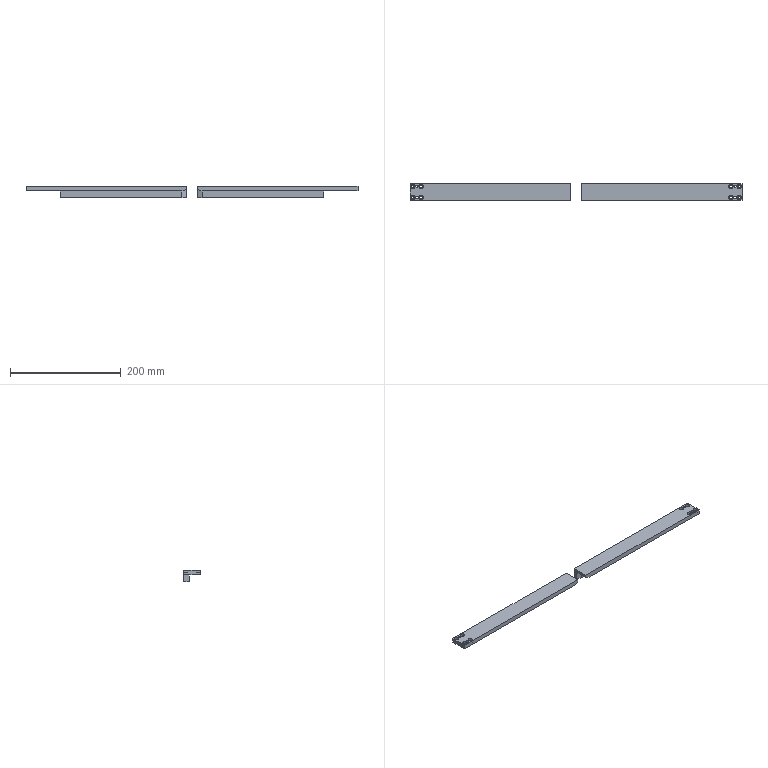NC program | NX | posted with a generic post | part box 600 x 30 x 20 mm
Lines 377 to 1170 of 2978:
(ZLEVEL_PROFILE_COPY_1_COPY , TOOL : D3)
N716 T20 M6
N718 G54
N720 G17 G0 G90 X-132.849 Y9.713 S7000 M3
N722 G43 Z30. H20
N724 Z1.
N726 G94 G1 X-132.821 Y9.67 Z0.997 F1000.
N728 X-132.617 Y9.555 Z0.985
N730 X-132.383 Z0.973
N732 X-132.179 Y9.67 Z0.961
N734 X-132.073 Y9.829 Z0.951
N736 X-132.04 Y10. Z0.941
N738 X-132.073 Y10.171 Z0.932
N740 X-132.179 Y10.33 Z0.922
N742 X-132.405 Y10.45 Z0.909
N744 X-132.595 Z0.899
N746 X-132.671 Y10.427 Z0.895
N748 X-132.83 Y10.321 Z0.885
N750 X-132.951 Y10.089 Z0.871
N752 X-132.927 Y9.829 Z0.857
N754 X-132.821 Y9.67 Z0.847
N756 X-132.617 Y9.555 Z0.835
N758 X-132.383 Z0.823
N760 X-132.179 Y9.67 Z0.811
N762 X-132.073 Y9.829 Z0.801
N764 X-132.04 Y10. Z0.791
N766 X-132.073 Y10.171 Z0.782
N768 X-132.179 Y10.33 Z0.772
N770 X-132.405 Y10.45 Z0.759
N772 X-132.595 Z0.749
N774 X-132.671 Y10.427 Z0.745
N776 X-132.83 Y10.321 Z0.735
N778 X-132.951 Y10.089 Z0.721
N780 X-132.927 Y9.829 Z0.707
N782 X-132.821 Y9.67 Z0.697
N784 X-132.617 Y9.555 Z0.685
N786 X-132.383 Z0.673
N788 X-132.179 Y9.67 Z0.66
N790 X-132.073 Y9.829 Z0.65
N792 X-132.04 Y10. Z0.641
N794 X-132.073 Y10.171 Z0.632
N796 X-132.179 Y10.33 Z0.622
N798 X-132.405 Y10.45 Z0.609
N800 X-132.595 Z0.599
N802 X-132.671 Y10.427 Z0.595
N804 X-132.83 Y10.321 Z0.585
N806 X-132.951 Y10.089 Z0.571
N808 X-132.927 Y9.829 Z0.557
N810 X-132.821 Y9.67 Z0.547
N812 X-132.617 Y9.555 Z0.535
N814 X-132.383 Z0.523
N816 X-132.179 Y9.67 Z0.51
N818 X-132.073 Y9.829 Z0.5
N820 X-132.04 Y10. Z0.491
N822 X-132.073 Y10.171 Z0.482
N824 X-132.179 Y10.33 Z0.472
N826 X-132.405 Y10.45 Z0.459
N828 X-132.595 Z0.449
N830 X-132.671 Y10.427 Z0.445
N832 X-132.83 Y10.321 Z0.435
N834 X-132.951 Y10.089 Z0.421
N836 X-132.927 Y9.829 Z0.407
N838 X-132.821 Y9.67 Z0.397
N840 X-132.617 Y9.555 Z0.385
N842 X-132.383 Z0.373
N844 X-132.179 Y9.67 Z0.36
N846 X-132.073 Y9.829 Z0.35
N848 X-132.04 Y10. Z0.341
N850 X-132.073 Y10.171 Z0.332
N852 X-132.179 Y10.33 Z0.322
N854 X-132.405 Y10.45 Z0.309
N856 X-132.595 Z0.299
N858 X-132.671 Y10.427 Z0.295
N860 X-132.83 Y10.321 Z0.285
N862 X-132.951 Y10.089 Z0.271
N864 X-132.927 Y9.829 Z0.257
N866 X-132.821 Y9.67 Z0.247
N868 X-132.617 Y9.555 Z0.235
N870 X-132.383 Z0.223
N872 X-132.179 Y9.67 Z0.21
N874 X-132.073 Y9.829 Z0.2
N876 X-132.04 Y10. Z0.191
N878 X-132.073 Y10.171 Z0.182
N880 X-132.179 Y10.33 Z0.172
N882 X-132.405 Y10.45 Z0.159
N884 X-132.595 Z0.149
N886 X-132.671 Y10.427 Z0.145
N888 X-132.83 Y10.321 Z0.135
N890 X-132.951 Y10.089 Z0.121
N892 X-132.927 Y9.829 Z0.107
N894 X-132.821 Y9.67 Z0.097
N896 X-132.617 Y9.555 Z0.085
N898 X-132.383 Z0.073
N900 X-132.179 Y9.67 Z0.06
N902 X-132.073 Y9.829 Z0.05
N904 X-132.04 Y10. Z0.041
N906 X-132.073 Y10.171 Z0.032
N908 X-132.179 Y10.33 Z0.022
N910 X-132.405 Y10.45 Z0.009
N912 X-132.595 Z-0.001
N914 X-132.671 Y10.427 Z-0.005
N916 X-132.83 Y10.321 Z-0.015
N918 X-132.951 Y10.089 Z-0.029
N920 X-132.927 Y9.829 Z-0.043
N922 X-132.821 Y9.67 Z-0.053
N924 X-132.617 Y9.555 Z-0.065
N926 X-132.383 Z-0.077
N928 X-132.179 Y9.67 Z-0.09
N930 X-132.073 Y9.829 Z-0.1
N932 X-132.04 Y10. Z-0.109
N934 X-132.073 Y10.171 Z-0.118
N936 X-132.179 Y10.33 Z-0.128
N938 X-132.405 Y10.45 Z-0.141
N940 X-132.595 Z-0.151
N942 X-132.671 Y10.427 Z-0.155
N944 X-132.83 Y10.321 Z-0.165
N946 X-132.951 Y10.089 Z-0.179
N948 X-132.927 Y9.829 Z-0.193
N950 X-132.821 Y9.67 Z-0.203
N952 X-132.617 Y9.555 Z-0.215
N954 X-132.383 Z-0.227
N956 X-132.179 Y9.67 Z-0.24
N958 X-132.073 Y9.829 Z-0.25
N960 X-132.04 Y10. Z-0.259
N962 X-132.073 Y10.171 Z-0.268
N964 X-132.179 Y10.33 Z-0.278
N966 X-132.405 Y10.45 Z-0.291
N968 X-132.5 Z-0.296
N970 G3 X-132.95 Y10. R0.45 F1300.
N972 X-132.5 Y10.45 R-0.45
N974 G1 X-132.596 Y10.433 Z-0.31
N976 X-132.669 Y10.41 Z-0.321
N978 X-132.721 Y10.383 Z-0.329
N980 X-132.8 Y10.325 Z-0.343
N982 X-132.851 Y10.269 Z-0.354
N984 X-132.883 Y10.221 Z-0.362
N986 X-132.921 Y10.132 Z-0.376
N988 X-132.936 Y10.086 Z-0.383
N990 X-132.944 Y10. Z-0.395
N992 X-132.933 Y9.91 Z-0.408
N994 X-132.911 Y9.837 Z-0.419
N996 X-132.883 Y9.779 Z-0.428
N998 X-132.828 Y9.702 Z-0.441
N1000 X-132.795 Y9.67 Z-0.448
N1002 X-132.771 Y9.651 Z-0.452
N1004 X-132.721 Y9.617 Z-0.461
N1006 X-132.632 Y9.579 Z-0.474
N1008 X-132.587 Y9.564 Z-0.481
N1010 X-132.5 Y9.556 Z-0.494
N1012 X-132.412 Y9.565 Z-0.506
N1014 X-132.339 Y9.587 Z-0.517
N1016 X-132.279 Y9.617 Z-0.527
N1018 X-132.197 Y9.678 Z-0.541
N1020 X-132.163 Y9.715 Z-0.548
N1022 X-132.11 Y9.775 Z-0.56
N1024 X-132.084 Y9.828 Z-0.568
N1026 X-132.065 Y9.884 Z-0.576
N1028 X-132.054 Y9.941 Z-0.584
N1030 X-132.05 Y10. Z-0.593
N1032 G3 X-132.5 Y10.45 R0.45
N1034 G1 X-132.596 Y10.433 Z-0.606
N1036 X-132.669 Y10.41 Z-0.617
N1038 X-132.721 Y10.383 Z-0.626
N1040 X-132.8 Y10.325 Z-0.639
N1042 X-132.851 Y10.269 Z-0.65
N1044 X-132.883 Y10.221 Z-0.658
N1046 X-132.921 Y10.132 Z-0.672
N1048 X-132.936 Y10.086 Z-0.679
N1050 X-132.944 Y10. Z-0.691
N1052 X-132.933 Y9.91 Z-0.704
N1054 X-132.911 Y9.837 Z-0.715
N1056 X-132.883 Y9.779 Z-0.724
N1058 X-132.827 Y9.702 Z-0.738
N1060 X-132.795 Y9.67 Z-0.744
N1062 X-132.771 Y9.651 Z-0.748
N1064 X-132.721 Y9.617 Z-0.757
N1066 X-132.632 Y9.579 Z-0.771
N1068 X-132.587 Y9.564 Z-0.778
N1070 X-132.5 Y9.556 Z-0.79
N1072 X-132.412 Y9.565 Z-0.803
N1074 X-132.339 Y9.587 Z-0.814
N1076 X-132.279 Y9.617 Z-0.823
N1078 X-132.197 Y9.678 Z-0.837
N1080 X-132.163 Y9.715 Z-0.845
N1082 X-132.11 Y9.775 Z-0.856
N1084 X-132.084 Y9.828 Z-0.864
N1086 X-132.065 Y9.884 Z-0.872
N1088 X-132.054 Y9.941 Z-0.881
N1090 X-132.05 Y10. Z-0.889
N1092 G3 X-132.5 Y10.45 R0.45
N1094 G1 X-132.596 Y10.433 Z-0.902
N1096 X-132.669 Y10.41 Z-0.913
N1098 X-132.721 Y10.383 Z-0.922
N1100 X-132.8 Y10.325 Z-0.936
N1102 X-132.851 Y10.269 Z-0.946
N1104 X-132.883 Y10.221 Z-0.955
N1106 X-132.921 Y10.132 Z-0.968
N1108 X-132.936 Y10.086 Z-0.975
N1110 X-132.944 Y10. Z-0.988
N1112 X-132.933 Y9.91 Z-1.
N1114 X-132.911 Y9.837 Z-1.011
N1116 X-132.883 Y9.779 Z-1.021
N1118 X-132.827 Y9.702 Z-1.034
N1120 X-132.795 Y9.67 Z-1.04
N1122 X-132.771 Y9.651 Z-1.045
N1124 X-132.721 Y9.617 Z-1.053
N1126 X-132.632 Y9.579 Z-1.067
N1128 X-132.587 Y9.564 Z-1.074
N1130 X-132.5 Y9.556 Z-1.086
N1132 X-132.412 Y9.565 Z-1.099
N1134 X-132.339 Y9.587 Z-1.11
N1136 X-132.279 Y9.617 Z-1.119
N1138 X-132.197 Y9.678 Z-1.134
N1140 X-132.163 Y9.715 Z-1.141
N1142 X-132.11 Y9.775 Z-1.152
N1144 X-132.084 Y9.828 Z-1.16
N1146 X-132.065 Y9.884 Z-1.169
N1148 X-132.054 Y9.941 Z-1.177
N1150 X-132.05 Y10. Z-1.185
N1152 G3 X-132.5 Y10.45 R0.45
N1154 G1 X-132.596 Y10.433 Z-1.199
N1156 X-132.669 Y10.41 Z-1.21
N1158 X-132.721 Y10.383 Z-1.218
N1160 X-132.8 Y10.325 Z-1.232
N1162 X-132.851 Y10.269 Z-1.243
N1164 X-132.883 Y10.221 Z-1.251
N1166 X-132.921 Y10.132 Z-1.265
N1168 X-132.936 Y10.086 Z-1.271
N1170 X-132.944 Y10. Z-1.284
N1172 X-132.933 Y9.91 Z-1.297
N1174 X-132.911 Y9.837 Z-1.308
N1176 X-132.883 Y9.779 Z-1.317
N1178 X-132.827 Y9.702 Z-1.33
N1180 X-132.795 Y9.67 Z-1.337
N1182 X-132.771 Y9.651 Z-1.341
N1184 X-132.721 Y9.617 Z-1.35
N1186 X-132.632 Y9.579 Z-1.363
N1188 X-132.587 Y9.564 Z-1.37
N1190 X-132.5 Y9.556 Z-1.383
N1192 X-132.412 Y9.565 Z-1.395
N1194 X-132.339 Y9.587 Z-1.406
N1196 X-132.279 Y9.617 Z-1.416
N1198 X-132.197 Y9.678 Z-1.43
N1200 X-132.163 Y9.715 Z-1.437
N1202 X-132.11 Y9.775 Z-1.449
N1204 X-132.084 Y9.828 Z-1.457
N1206 X-132.065 Y9.884 Z-1.465
N1208 X-132.054 Y9.941 Z-1.473
N1210 X-132.05 Y10. Z-1.481
N1212 G3 X-132.5 Y10.45 R0.45
N1214 G1 X-132.596 Y10.433 Z-1.495
N1216 X-132.669 Y10.41 Z-1.506
N1218 X-132.721 Y10.383 Z-1.514
N1220 X-132.8 Y10.325 Z-1.528
N1222 X-132.851 Y10.269 Z-1.539
N1224 X-132.883 Y10.221 Z-1.547
N1226 X-132.921 Y10.132 Z-1.561
N1228 X-132.936 Y10.086 Z-1.568
N1230 X-132.944 Y10. Z-1.58
N1232 X-132.933 Y9.91 Z-1.593
N1234 X-132.911 Y9.837 Z-1.604
N1236 X-132.883 Y9.779 Z-1.613
N1238 X-132.827 Y9.702 Z-1.626
N1240 X-132.795 Y9.67 Z-1.633
N1242 X-132.771 Y9.651 Z-1.637
N1244 X-132.721 Y9.617 Z-1.646
N1246 X-132.632 Y9.579 Z-1.66
N1248 X-132.587 Y9.564 Z-1.666
N1250 X-132.5 Y9.556 Z-1.679
N1252 X-132.412 Y9.565 Z-1.691
N1254 X-132.339 Y9.587 Z-1.702
N1256 X-132.279 Y9.617 Z-1.712
N1258 X-132.197 Y9.678 Z-1.726
N1260 X-132.163 Y9.715 Z-1.733
N1262 X-132.11 Y9.775 Z-1.745
N1264 X-132.084 Y9.828 Z-1.753
N1266 X-132.065 Y9.884 Z-1.761
N1268 X-132.054 Y9.941 Z-1.77
N1270 X-132.05 Y10. Z-1.778
N1272 G3 X-132.5 Y10.45 R0.45
N1274 G1 X-132.596 Y10.433 Z-1.791
N1276 X-132.669 Y10.41 Z-1.802
N1278 X-132.721 Y10.383 Z-1.811
N1280 X-132.8 Y10.325 Z-1.824
N1282 X-132.851 Y10.269 Z-1.835
N1284 X-132.883 Y10.221 Z-1.844
N1286 X-132.921 Y10.132 Z-1.857
N1288 X-132.936 Y10.086 Z-1.864
N1290 X-132.944 Y10. Z-1.877
N1292 X-132.933 Y9.91 Z-1.889
N1294 X-132.911 Y9.837 Z-1.9
N1296 X-132.883 Y9.779 Z-1.909
N1298 X-132.827 Y9.702 Z-1.923
N1300 X-132.795 Y9.67 Z-1.929
N1302 X-132.771 Y9.651 Z-1.934
N1304 X-132.721 Y9.617 Z-1.942
N1306 X-132.632 Y9.579 Z-1.956
N1308 X-132.587 Y9.564 Z-1.963
N1310 X-132.5 Y9.556 Z-1.975
N1312 X-132.412 Y9.565 Z-1.988
N1314 X-132.339 Y9.587 Z-1.999
N1316 X-132.279 Y9.617 Z-2.008
N1318 X-132.197 Y9.678 Z-2.023
N1320 X-132.163 Y9.715 Z-2.03
N1322 X-132.11 Y9.775 Z-2.041
N1324 X-132.084 Y9.828 Z-2.049
N1326 X-132.065 Y9.884 Z-2.058
N1328 X-132.054 Y9.941 Z-2.066
N1330 X-132.05 Y10. Z-2.074
N1332 G3 X-132.5 Y10.45 R0.45
N1334 G1 X-132.596 Y10.433 Z-2.088
N1336 X-132.669 Y10.41 Z-2.099
N1338 X-132.721 Y10.383 Z-2.107
N1340 X-132.8 Y10.325 Z-2.121
N1342 X-132.851 Y10.269 Z-2.132
N1344 X-132.883 Y10.221 Z-2.14
N1346 X-132.921 Y10.132 Z-2.154
N1348 X-132.936 Y10.086 Z-2.16
N1350 X-132.944 Y10. Z-2.173
N1352 X-132.933 Y9.91 Z-2.186
N1354 X-132.911 Y9.837 Z-2.197
N1356 X-132.883 Y9.779 Z-2.206
N1358 X-132.827 Y9.702 Z-2.219
N1360 X-132.795 Y9.67 Z-2.226
N1362 X-132.771 Y9.651 Z-2.23
N1364 X-132.721 Y9.617 Z-2.239
N1366 X-132.632 Y9.579 Z-2.252
N1368 X-132.587 Y9.565 Z-2.259
N1370 X-132.5 Y9.556 Z-2.272
N1372 X-132.412 Y9.565 Z-2.284
N1374 X-132.339 Y9.587 Z-2.295
N1376 X-132.279 Y9.617 Z-2.305
N1378 X-132.197 Y9.678 Z-2.319
N1380 X-132.163 Y9.715 Z-2.326
N1382 X-132.11 Y9.775 Z-2.337
N1384 X-132.084 Y9.828 Z-2.346
N1386 X-132.065 Y9.884 Z-2.354
N1388 X-132.054 Y9.941 Z-2.362
N1390 X-132.05 Y10. Z-2.37
N1392 G3 X-132.5 Y10.45 R0.45
N1394 G1 X-132.596 Y10.433 Z-2.384
N1396 X-132.669 Y10.41 Z-2.395
N1398 X-132.721 Y10.383 Z-2.403
N1400 X-132.8 Y10.325 Z-2.417
N1402 X-132.851 Y10.269 Z-2.428
N1404 X-132.883 Y10.221 Z-2.436
N1406 X-132.921 Y10.132 Z-2.45
N1408 X-132.936 Y10.086 Z-2.457
N1410 X-132.944 Y10. Z-2.469
N1412 X-132.933 Y9.91 Z-2.482
N1414 X-132.911 Y9.837 Z-2.493
N1416 X-132.883 Y9.779 Z-2.502
N1418 X-132.827 Y9.702 Z-2.515
N1420 X-132.795 Y9.67 Z-2.522
N1422 X-132.771 Y9.651 Z-2.526
N1424 X-132.721 Y9.617 Z-2.535
N1426 X-132.632 Y9.579 Z-2.549
N1428 X-132.587 Y9.565 Z-2.555
N1430 X-132.5 Y9.556 Z-2.568
N1432 X-132.412 Y9.565 Z-2.58
N1434 X-132.339 Y9.587 Z-2.591
N1436 X-132.279 Y9.617 Z-2.601
N1438 X-132.197 Y9.678 Z-2.615
N1440 X-132.163 Y9.715 Z-2.622
N1442 X-132.11 Y9.775 Z-2.634
N1444 X-132.084 Y9.828 Z-2.642
N1446 X-132.065 Y9.884 Z-2.65
N1448 X-132.054 Y9.941 Z-2.658
N1450 X-132.05 Y10. Z-2.667
N1452 G3 X-132.5 Y10.45 R0.45
N1454 G1 X-132.596 Y10.433 Z-2.68
N1456 X-132.669 Y10.41 Z-2.691
N1458 X-132.721 Y10.383 Z-2.7
N1460 X-132.8 Y10.325 Z-2.713
N1462 X-132.851 Y10.269 Z-2.724
N1464 X-132.883 Y10.221 Z-2.733
N1466 X-132.921 Y10.132 Z-2.746
N1468 X-132.936 Y10.086 Z-2.753
N1470 X-132.944 Y10. Z-2.765
N1472 X-132.933 Y9.91 Z-2.778
N1474 X-132.911 Y9.837 Z-2.789
N1476 X-132.883 Y9.779 Z-2.798
N1478 X-132.827 Y9.702 Z-2.812
N1480 X-132.795 Y9.67 Z-2.818
N1482 X-132.771 Y9.651 Z-2.823
N1484 X-132.721 Y9.617 Z-2.831
N1486 X-132.632 Y9.579 Z-2.845
N1488 X-132.587 Y9.565 Z-2.852
N1490 X-132.5 Y9.556 Z-2.864
N1492 X-132.412 Y9.565 Z-2.877
N1494 X-132.339 Y9.587 Z-2.888
N1496 X-132.279 Y9.617 Z-2.897
N1498 X-132.197 Y9.678 Z-2.911
N1500 X-132.163 Y9.715 Z-2.919
N1502 X-132.11 Y9.775 Z-2.93
N1504 X-132.084 Y9.828 Z-2.938
N1506 X-132.065 Y9.884 Z-2.947
N1508 X-132.054 Y9.941 Z-2.955
N1510 X-132.05 Y10. Z-2.963
N1512 G3 X-132.5 Y10.45 R0.45
N1514 G1 X-132.596 Y10.433 Z-2.977
N1516 X-132.669 Y10.41 Z-2.988
N1518 X-132.721 Y10.383 Z-2.996
N1520 X-132.8 Y10.325 Z-3.01
N1522 X-132.851 Y10.269 Z-3.021
N1524 X-132.883 Y10.221 Z-3.029
N1526 X-132.921 Y10.132 Z-3.042
N1528 X-132.936 Y10.086 Z-3.049
N1530 X-132.944 Y10. Z-3.062
N1532 X-132.933 Y9.91 Z-3.074
N1534 X-132.911 Y9.837 Z-3.085
N1536 X-132.883 Y9.779 Z-3.095
N1538 X-132.827 Y9.702 Z-3.108
N1540 X-132.795 Y9.67 Z-3.115
N1542 X-132.771 Y9.651 Z-3.119
N1544 X-132.721 Y9.617 Z-3.128
N1546 X-132.632 Y9.579 Z-3.141
N1548 X-132.587 Y9.565 Z-3.148
N1550 X-132.5 Y9.556 Z-3.16
N1552 X-132.412 Y9.565 Z-3.173
N1554 X-132.339 Y9.587 Z-3.184
N1556 X-132.279 Y9.617 Z-3.193
N1558 X-132.197 Y9.678 Z-3.208
N1560 X-132.163 Y9.715 Z-3.215
N1562 X-132.11 Y9.775 Z-3.226
N1564 X-132.084 Y9.828 Z-3.235
N1566 X-132.065 Y9.884 Z-3.243
N1568 X-132.054 Y9.941 Z-3.251
N1570 X-132.05 Y10. Z-3.259
N1572 G3 X-132.5 Y10.45 R0.45
N1574 G1 X-132.596 Y10.433 Z-3.273
N1576 X-132.669 Y10.41 Z-3.284
N1578 X-132.721 Y10.383 Z-3.292
N1580 X-132.8 Y10.325 Z-3.306
N1582 X-132.851 Y10.269 Z-3.317
N1584 X-132.883 Y10.221 Z-3.325
N1586 X-132.921 Y10.132 Z-3.339
N1588 X-132.936 Y10.086 Z-3.346
N1590 X-132.944 Y10. Z-3.358
N1592 X-132.933 Y9.91 Z-3.371
N1594 X-132.911 Y9.837 Z-3.382
N1596 X-132.883 Y9.779 Z-3.391
N1598 X-132.827 Y9.702 Z-3.404
N1600 X-132.795 Y9.67 Z-3.411
N1602 X-132.771 Y9.651 Z-3.415
N1604 X-132.721 Y9.617 Z-3.424
N1606 X-132.632 Y9.579 Z-3.437
N1608 X-132.587 Y9.565 Z-3.444
N1610 X-132.5 Y9.556 Z-3.457
N1612 X-132.412 Y9.565 Z-3.469
N1614 X-132.339 Y9.587 Z-3.48
N1616 X-132.279 Y9.617 Z-3.49
N1618 X-132.197 Y9.678 Z-3.504
N1620 X-132.163 Y9.715 Z-3.511
N1622 X-132.11 Y9.775 Z-3.523
N1624 X-132.084 Y9.828 Z-3.531
N1626 X-132.065 Y9.884 Z-3.539
N1628 X-132.054 Y9.941 Z-3.547
N1630 X-132.05 Y10. Z-3.556
N1632 G3 X-132.5 Y10.45 R0.45
N1634 G1 X-132.596 Y10.433 Z-3.569
N1636 X-132.669 Y10.41 Z-3.58
N1638 X-132.721 Y10.383 Z-3.588
N1640 X-132.8 Y10.325 Z-3.602
N1642 X-132.851 Y10.269 Z-3.613
N1644 X-132.883 Y10.221 Z-3.621
N1646 X-132.921 Y10.132 Z-3.635
N1648 X-132.936 Y10.086 Z-3.642
N1650 X-132.944 Y10. Z-3.654
N1652 X-132.933 Y9.91 Z-3.667
N1654 X-132.911 Y9.837 Z-3.678
N1656 X-132.883 Y9.779 Z-3.687
N1658 X-132.827 Y9.702 Z-3.7
N1660 X-132.795 Y9.67 Z-3.707
N1662 X-132.771 Y9.651 Z-3.711
N1664 X-132.721 Y9.617 Z-3.72
N1666 X-132.632 Y9.579 Z-3.734
N1668 X-132.587 Y9.565 Z-3.74
N1670 X-132.5 Y9.556 Z-3.753
N1672 X-132.412 Y9.565 Z-3.765
N1674 X-132.339 Y9.587 Z-3.776
N1676 X-132.279 Y9.617 Z-3.786
N1678 X-132.197 Y9.678 Z-3.8
N1680 X-132.163 Y9.715 Z-3.807
N1682 X-132.11 Y9.775 Z-3.819
N1684 X-132.084 Y9.828 Z-3.827
N1686 X-132.065 Y9.884 Z-3.835
N1688 X-132.054 Y9.941 Z-3.844
N1690 X-132.05 Y10. Z-3.852
N1692 G3 X-132.5 Y10.45 R0.45
N1694 G1 X-132.596 Y10.433 Z-3.865
N1696 X-132.669 Y10.41 Z-3.876
N1698 X-132.721 Y10.383 Z-3.885
N1700 X-132.8 Y10.325 Z-3.898
N1702 X-132.851 Y10.269 Z-3.909
N1704 X-132.883 Y10.221 Z-3.918
N1706 X-132.921 Y10.132 Z-3.931
N1708 X-132.936 Y10.086 Z-3.938
N1710 X-132.944 Y10. Z-3.951
N1712 X-132.935 Y9.909 Z-3.963
N1714 X-132.911 Y9.837 Z-3.974
N1716 X-132.883 Y9.779 Z-3.984
N1718 X-132.827 Y9.702 Z-3.997
N1720 X-132.795 Y9.67 Z-4.003
N1722 X-132.771 Y9.651 Z-4.008
N1724 X-132.721 Y9.617 Z-4.016
N1726 X-132.632 Y9.579 Z-4.03
N1728 X-132.587 Y9.565 Z-4.037
N1730 X-132.5 Y9.556 Z-4.049
N1732 X-132.412 Y9.565 Z-4.062
N1734 X-132.339 Y9.587 Z-4.073
N1736 X-132.279 Y9.617 Z-4.082
N1738 X-132.197 Y9.678 Z-4.097
N1740 X-132.163 Y9.715 Z-4.104
N1742 X-132.11 Y9.775 Z-4.115
N1744 X-132.084 Y9.828 Z-4.123
N1746 X-132.065 Y9.884 Z-4.132
N1748 X-132.054 Y9.941 Z-4.14
N1750 X-132.05 Y10. Z-4.148
N1752 G3 X-132.5 Y10.45 R0.45
N1754 G1 X-132.596 Y10.433 Z-4.162
N1756 X-132.669 Y10.41 Z-4.173
N1758 X-132.721 Y10.383 Z-4.181
N1760 X-132.8 Y10.325 Z-4.195
N1762 X-132.851 Y10.269 Z-4.206
N1764 X-132.883 Y10.221 Z-4.214
N1766 X-132.921 Y10.132 Z-4.228
N1768 X-132.936 Y10.086 Z-4.234
N1770 X-132.944 Y10. Z-4.247
N1772 X-132.935 Y9.909 Z-4.26
N1774 X-132.911 Y9.837 Z-4.271
N1776 X-132.883 Y9.779 Z-4.28
N1778 X-132.827 Y9.702 Z-4.293
N1780 X-132.795 Y9.67 Z-4.3
N1782 X-132.771 Y9.651 Z-4.304
N1784 X-132.721 Y9.617 Z-4.313
N1786 X-132.632 Y9.579 Z-4.326
N1788 X-132.587 Y9.565 Z-4.333
N1790 X-132.5 Y9.556 Z-4.346
N1792 X-132.412 Y9.565 Z-4.358
N1794 X-132.339 Y9.587 Z-4.369
N1796 X-132.279 Y9.617 Z-4.379
N1798 X-132.197 Y9.678 Z-4.393
N1800 X-132.163 Y9.715 Z-4.4
N1802 X-132.11 Y9.775 Z-4.412
N1804 X-132.084 Y9.828 Z-4.42
N1806 X-132.065 Y9.884 Z-4.428
N1808 X-132.054 Y9.941 Z-4.436
N1810 X-132.05 Y10. Z-4.444
N1812 G3 X-132.5 Y10.45 R0.45
N1814 G1 X-132.596 Y10.433 Z-4.458
N1816 X-132.669 Y10.41 Z-4.469
N1818 X-132.721 Y10.383 Z-4.477
N1820 X-132.8 Y10.325 Z-4.491
N1822 X-132.851 Y10.269 Z-4.502
N1824 X-132.883 Y10.221 Z-4.51
N1826 X-132.921 Y10.132 Z-4.524
N1828 X-132.936 Y10.086 Z-4.531
N1830 X-132.944 Y10. Z-4.543
N1832 X-132.935 Y9.909 Z-4.556
N1834 X-132.911 Y9.837 Z-4.567
N1836 X-132.883 Y9.779 Z-4.576
N1838 X-132.827 Y9.702 Z-4.589
N1840 X-132.795 Y9.67 Z-4.596
N1842 X-132.771 Y9.651 Z-4.6
N1844 X-132.721 Y9.617 Z-4.609
N1846 X-132.632 Y9.579 Z-4.623
N1848 X-132.587 Y9.565 Z-4.629
N1850 X-132.5 Y9.556 Z-4.642
N1852 X-132.412 Y9.565 Z-4.654
N1854 X-132.339 Y9.587 Z-4.665
N1856 X-132.279 Y9.617 Z-4.675
N1858 X-132.197 Y9.678 Z-4.689
N1860 X-132.163 Y9.715 Z-4.696
N1862 X-132.11 Y9.775 Z-4.708
N1864 X-132.084 Y9.828 Z-4.716
N1866 X-132.065 Y9.884 Z-4.724
N1868 X-132.054 Y9.941 Z-4.733
N1870 X-132.05 Y10. Z-4.741
N1872 G3 X-132.5 Y10.45 R0.45
N1874 G1 X-132.596 Y10.433 Z-4.754
N1876 X-132.669 Y10.41 Z-4.765
N1878 X-132.721 Y10.383 Z-4.774
N1880 X-132.8 Y10.325 Z-4.787
N1882 X-132.851 Y10.269 Z-4.798
N1884 X-132.883 Y10.221 Z-4.807
N1886 X-132.921 Y10.132 Z-4.82
N1888 X-132.936 Y10.086 Z-4.827
N1890 X-132.944 Y10. Z-4.84
N1892 X-132.935 Y9.909 Z-4.852
N1894 X-132.911 Y9.837 Z-4.863
N1896 X-132.883 Y9.779 Z-4.872
N1898 X-132.827 Y9.703 Z-4.886
N1900 X-132.795 Y9.67 Z-4.892
N1902 X-132.771 Y9.651 Z-4.897
N1904 X-132.721 Y9.617 Z-4.905
N1906 X-132.632 Y9.579 Z-4.919
N1908 X-132.587 Y9.565 Z-4.926
N1910 X-132.5 Y9.556 Z-4.938
N1912 X-132.412 Y9.565 Z-4.951
N1914 X-132.339 Y9.587 Z-4.962
N1916 X-132.279 Y9.617 Z-4.971
N1918 X-132.197 Y9.678 Z-4.985
N1920 X-132.163 Y9.715 Z-4.993
N1922 X-132.11 Y9.775 Z-5.004
N1924 X-132.084 Y9.828 Z-5.012
N1926 X-132.065 Y9.884 Z-5.021
N1928 X-132.054 Y9.941 Z-5.029
N1930 X-132.05 Y10. Z-5.037
N1932 G3 X-132.5 Y10.45 R0.45
N1934 G1 X-132.595 Y10.433 Z-5.051
N1936 X-132.669 Y10.41 Z-5.062
N1938 X-132.721 Y10.383 Z-5.07
N1940 X-132.8 Y10.325 Z-5.084
N1942 X-132.851 Y10.269 Z-5.095
N1944 X-132.883 Y10.221 Z-5.103
N1946 X-132.921 Y10.132 Z-5.116
N1948 X-132.936 Y10.086 Z-5.123
N1950 X-132.944 Y10. Z-5.136
N1952 X-132.935 Y9.909 Z-5.149
N1954 X-132.911 Y9.837 Z-5.16
N1956 X-132.883 Y9.779 Z-5.169
N1958 X-132.827 Y9.703 Z-5.182
N1960 X-132.795 Y9.67 Z-5.189
N1962 X-132.771 Y9.651 Z-5.193
N1964 X-132.721 Y9.617 Z-5.202
N1966 X-132.632 Y9.579 Z-5.215
N1968 X-132.587 Y9.565 Z-5.222
N1970 X-132.5 Y9.556 Z-5.235
N1972 X-132.412 Y9.565 Z-5.247
N1974 X-132.339 Y9.587 Z-5.258
N1976 X-132.279 Y9.617 Z-5.267
N1978 X-132.197 Y9.678 Z-5.282
N1980 X-132.163 Y9.715 Z-5.289
N1982 X-132.11 Y9.775 Z-5.3
N1984 X-132.084 Y9.828 Z-5.309
N1986 X-132.065 Y9.884 Z-5.317
N1988 X-132.054 Y9.941 Z-5.325
N1990 X-132.05 Y10. Z-5.333
N1992 G3 X-132.5 Y10.45 R0.45
N1994 G1 X-132.595 Y10.433 Z-5.347
N1996 X-132.669 Y10.41 Z-5.358
N1998 X-132.721 Y10.383 Z-5.366
N2000 X-132.8 Y10.325 Z-5.38
N2002 X-132.851 Y10.269 Z-5.391
N2004 X-132.883 Y10.221 Z-5.399
N2006 X-132.921 Y10.132 Z-5.413
N2008 X-132.936 Y10.086 Z-5.42
N2010 X-132.944 Y10. Z-5.432
N2012 X-132.935 Y9.909 Z-5.445
N2014 X-132.911 Y9.837 Z-5.456
N2016 X-132.883 Y9.779 Z-5.465
N2018 X-132.827 Y9.703 Z-5.478
N2020 X-132.795 Y9.67 Z-5.485
N2022 X-132.771 Y9.651 Z-5.489
N2024 X-132.721 Y9.617 Z-5.498
N2026 X-132.632 Y9.579 Z-5.511
N2028 X-132.587 Y9.565 Z-5.518
N2030 X-132.5 Y9.556 Z-5.531
N2032 X-132.412 Y9.565 Z-5.543
N2034 X-132.339 Y9.587 Z-5.554
N2036 X-132.279 Y9.617 Z-5.564
N2038 X-132.197 Y9.678 Z-5.578
N2040 X-132.163 Y9.715 Z-5.585
N2042 X-132.11 Y9.775 Z-5.597
N2044 X-132.084 Y9.828 Z-5.605
N2046 X-132.065 Y9.884 Z-5.613
N2048 X-132.054 Y9.941 Z-5.621
N2050 X-132.05 Y10. Z-5.63
N2052 G3 X-132.5 Y10.45 R0.45
N2054 G1 X-132.595 Y10.433 Z-5.643
N2056 X-132.669 Y10.41 Z-5.654
N2058 X-132.721 Y10.383 Z-5.663
N2060 X-132.8 Y10.325 Z-5.676
N2062 X-132.851 Y10.269 Z-5.687
N2064 X-132.883 Y10.221 Z-5.695
N2066 X-132.921 Y10.132 Z-5.709
N2068 X-132.936 Y10.086 Z-5.716
N2070 X-132.944 Y10. Z-5.728
N2072 X-132.935 Y9.909 Z-5.741
N2074 X-132.911 Y9.837 Z-5.752
N2076 X-132.883 Y9.779 Z-5.761
N2078 X-132.827 Y9.703 Z-5.775
N2080 X-132.795 Y9.67 Z-5.781
N2082 X-132.771 Y9.651 Z-5.786
N2084 X-132.721 Y9.617 Z-5.794
N2086 X-132.632 Y9.579 Z-5.808
N2088 X-132.587 Y9.565 Z-5.815
N2090 X-132.5 Y9.556 Z-5.827
N2092 X-132.412 Y9.565 Z-5.84
N2094 X-132.339 Y9.587 Z-5.851
N2096 X-132.279 Y9.617 Z-5.86
N2098 X-132.197 Y9.678 Z-5.874
N2100 X-132.163 Y9.715 Z-5.882
N2102 X-132.11 Y9.775 Z-5.893
N2104 X-132.084 Y9.828 Z-5.901
N2106 X-132.065 Y9.884 Z-5.909
N2108 X-132.054 Y9.941 Z-5.918
N2110 X-132.05 Y10. Z-5.926
N2112 G3 X-132.5 Y10.45 R0.45
N2114 G1 X-132.595 Y10.433 Z-5.939
N2116 X-132.669 Y10.41 Z-5.95
N2118 X-132.721 Y10.383 Z-5.959
N2120 X-132.8 Y10.325 Z-5.973
N2122 X-132.851 Y10.269 Z-5.984
N2124 X-132.883 Y10.221 Z-5.992
N2126 X-132.921 Y10.132 Z-6.005
N2128 X-132.936 Y10.086 Z-6.012
N2130 X-132.944 Y10. Z-6.025
N2132 X-132.935 Y9.909 Z-6.037
N2134 X-132.911 Y9.837 Z-6.048
N2136 X-132.883 Y9.779 Z-6.058
N2138 X-132.827 Y9.703 Z-6.071
N2140 X-132.795 Y9.67 Z-6.077
N2142 X-132.771 Y9.651 Z-6.082
N2144 X-132.721 Y9.617 Z-6.091
N2146 X-132.632 Y9.579 Z-6.104
N2148 X-132.587 Y9.565 Z-6.111
N2150 X-132.5 Y9.556 Z-6.123
N2152 X-132.412 Y9.565 Z-6.136
N2154 X-132.339 Y9.587 Z-6.147
N2156 X-132.279 Y9.617 Z-6.156
N2158 X-132.197 Y9.678 Z-6.171
N2160 X-132.163 Y9.715 Z-6.178
N2162 X-132.11 Y9.775 Z-6.189
N2164 X-132.084 Y9.828 Z-6.198
N2166 X-132.065 Y9.884 Z-6.206
N2168 X-132.054 Y9.941 Z-6.214
N2170 X-132.05 Y10. Z-6.222
N2172 G3 X-132.5 Y10.45 R0.45
N2174 G1 X-132.595 Y10.433 Z-6.236
N2176 X-132.669 Y10.41 Z-6.247
N2178 X-132.721 Y10.383 Z-6.255
N2180 X-132.8 Y10.325 Z-6.269
N2182 X-132.851 Y10.269 Z-6.28
N2184 X-132.883 Y10.221 Z-6.288
N2186 X-132.921 Y10.132 Z-6.302
N2188 X-132.936 Y10.086 Z-6.309
N2190 X-132.944 Y10. Z-6.321
N2192 X-132.935 Y9.909 Z-6.334
N2194 X-132.911 Y9.837 Z-6.345
N2196 X-132.883 Y9.779 Z-6.354
N2198 X-132.827 Y9.703 Z-6.367
N2200 X-132.795 Y9.67 Z-6.374
N2202 X-132.771 Y9.651 Z-6.378
N2204 X-132.721 Y9.617 Z-6.387
N2206 X-132.632 Y9.579 Z-6.4
N2208 X-132.587 Y9.565 Z-6.407
N2210 X-132.5 Y9.556 Z-6.42
N2212 X-132.412 Y9.565 Z-6.432
N2214 X-132.339 Y9.587 Z-6.443
N2216 X-132.279 Y9.617 Z-6.453
N2218 X-132.197 Y9.678 Z-6.467
N2220 X-132.163 Y9.715 Z-6.474
N2222 X-132.11 Y9.775 Z-6.486
N2224 X-132.084 Y9.828 Z-6.494
N2226 X-132.065 Y9.884 Z-6.502
N2228 X-132.054 Y9.941 Z-6.51
N2230 X-132.05 Y10. Z-6.519
N2232 G3 X-132.5 Y10.45 R0.45
N2234 G1 X-132.595 Y10.433 Z-6.532
N2236 X-132.669 Y10.41 Z-6.543
N2238 X-132.721 Y10.383 Z-6.551
N2240 X-132.8 Y10.325 Z-6.565
N2242 X-132.851 Y10.269 Z-6.576
N2244 X-132.883 Y10.221 Z-6.584
N2246 X-132.921 Y10.132 Z-6.598
N2248 X-132.936 Y10.086 Z-6.605
N2250 X-132.944 Y10. Z-6.617
N2252 X-132.935 Y9.909 Z-6.63
N2254 X-132.911 Y9.837 Z-6.641
N2256 X-132.883 Y9.779 Z-6.65
N2258 X-132.827 Y9.703 Z-6.663
N2260 X-132.795 Y9.67 Z-6.67
N2262 X-132.771 Y9.651 Z-6.674
N2264 X-132.721 Y9.617 Z-6.683
N2266 X-132.632 Y9.579 Z-6.697
N2268 X-132.587 Y9.565 Z-6.703
N2270 X-132.5 Y9.556 Z-6.716
N2272 X-132.412 Y9.565 Z-6.728
N2274 X-132.339 Y9.587 Z-6.739
N2276 X-132.279 Y9.617 Z-6.749
N2278 X-132.197 Y9.678 Z-6.763
N2280 X-132.163 Y9.715 Z-6.77
N2282 X-132.11 Y9.775 Z-6.782
N2284 X-132.084 Y9.828 Z-6.79
N2286 X-132.065 Y9.884 Z-6.798
N2288 X-132.054 Y9.941 Z-6.807
N2290 X-132.05 Y10. Z-6.815
N2292 G3 X-132.5 Y10.45 R0.45
N2294 G1 X-132.595 Y10.433 Z-6.828
N2296 X-132.669 Y10.41 Z-6.839